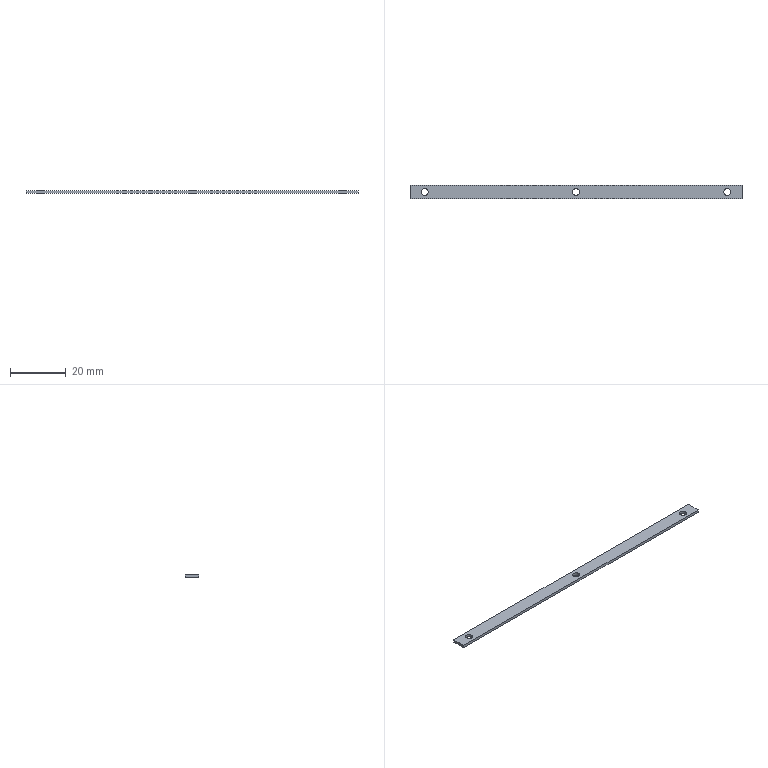Part | SolidWorks | features Cut 1, Extrusion 1 | 1 solid | 12 faces | box 119.31 x 4.994 x 1 mm | volume 581.134 mm3 | cylinder 6 | plane 6 | commonest cylinder face diameters 2.5 x6
STEP:
#1=CARTESIAN_POINT('',(-55.55,59.584,0.));
#2=VERTEX_POINT('',#1);
#3=CARTESIAN_POINT('',(-53.05,59.584,0.));
#4=VERTEX_POINT('',#3);
#5=CARTESIAN_POINT('',(-54.3,59.584,0.));
#6=DIRECTION('',(0.,0.,1.));
#7=DIRECTION('',(1.,0.,0.));
#8=AXIS2_PLACEMENT_3D('',#5,#6,#7);
#9=CIRCLE('',#8,1.25);
#10=EDGE_CURVE('',#2,#4,#9,.T.);
#11=ORIENTED_EDGE('',*,*,#10,.F.);
#12=CARTESIAN_POINT('',(-55.55,59.584,1.));
#13=VERTEX_POINT('',#12);
#14=CARTESIAN_POINT('',(-55.55,59.584,0.));
#15=DIRECTION('',(0.,0.,1.));
#16=VECTOR('',#15,1000.);
#17=LINE('',#14,#16);
#18=EDGE_CURVE('',#2,#13,#17,.T.);
#19=ORIENTED_EDGE('',*,*,#18,.T.);
#20=CARTESIAN_POINT('',(-53.05,59.584,1.));
#21=VERTEX_POINT('',#20);
#22=CARTESIAN_POINT('',(-54.3,59.584,1.));
#23=DIRECTION('',(0.,0.,1.));
#24=DIRECTION('',(1.,0.,0.));
#25=AXIS2_PLACEMENT_3D('',#22,#23,#24);
#26=CIRCLE('',#25,1.25);
#27=EDGE_CURVE('',#13,#21,#26,.T.);
#28=ORIENTED_EDGE('',*,*,#27,.T.);
#29=CARTESIAN_POINT('',(-53.05,59.584,0.));
#30=DIRECTION('',(0.,0.,1.));
#31=VECTOR('',#30,1000.);
#32=LINE('',#29,#31);
#33=EDGE_CURVE('',#4,#21,#32,.T.);
#34=ORIENTED_EDGE('',*,*,#33,.F.);
#35=EDGE_LOOP('',(#11,#19,#28,#34));
#36=FACE_OUTER_BOUND('',#35,.T.);
#37=CARTESIAN_POINT('',(-54.3,59.584,0.));
#38=DIRECTION('',(0.,0.,1.));
#39=DIRECTION('',(1.,0.,0.));
#40=AXIS2_PLACEMENT_3D('',#37,#38,#39);
#41=CYLINDRICAL_SURFACE('',#40,1.25);
#42=ADVANCED_FACE('',(#36),#41,.F.);
#43=CARTESIAN_POINT('',(-1.25,59.56,0.));
#44=VERTEX_POINT('',#43);
#45=CARTESIAN_POINT('',(1.25,59.56,0.));
#46=VERTEX_POINT('',#45);
#47=CARTESIAN_POINT('',(0.,59.56,0.));
#48=DIRECTION('',(0.,0.,1.));
#49=DIRECTION('',(1.,0.,0.));
#50=AXIS2_PLACEMENT_3D('',#47,#48,#49);
#51=CIRCLE('',#50,1.25);
#52=EDGE_CURVE('',#44,#46,#51,.T.);
#53=ORIENTED_EDGE('',*,*,#52,.F.);
#54=CARTESIAN_POINT('',(-1.25,59.56,1.));
#55=VERTEX_POINT('',#54);
#56=CARTESIAN_POINT('',(-1.25,59.56,0.));
#57=DIRECTION('',(0.,0.,1.));
#58=VECTOR('',#57,1000.);
#59=LINE('',#56,#58);
#60=EDGE_CURVE('',#44,#55,#59,.T.);
#61=ORIENTED_EDGE('',*,*,#60,.T.);
#62=CARTESIAN_POINT('',(1.25,59.56,1.));
#63=VERTEX_POINT('',#62);
#64=CARTESIAN_POINT('',(0.,59.56,1.));
#65=DIRECTION('',(0.,0.,1.));
#66=DIRECTION('',(1.,0.,0.));
#67=AXIS2_PLACEMENT_3D('',#64,#65,#66);
#68=CIRCLE('',#67,1.25);
#69=EDGE_CURVE('',#55,#63,#68,.T.);
#70=ORIENTED_EDGE('',*,*,#69,.T.);
#71=CARTESIAN_POINT('',(1.25,59.56,0.));
#72=DIRECTION('',(0.,0.,1.));
#73=VECTOR('',#72,1000.);
#74=LINE('',#71,#73);
#75=EDGE_CURVE('',#46,#63,#74,.T.);
#76=ORIENTED_EDGE('',*,*,#75,.F.);
#77=EDGE_LOOP('',(#53,#61,#70,#76));
#78=FACE_OUTER_BOUND('',#77,.T.);
#79=CARTESIAN_POINT('',(0.,59.56,0.));
#80=DIRECTION('',(0.,0.,1.));
#81=DIRECTION('',(1.,0.,0.));
#82=AXIS2_PLACEMENT_3D('',#79,#80,#81);
#83=CYLINDRICAL_SURFACE('',#82,1.25);
#84=ADVANCED_FACE('',(#78),#83,.F.);
#85=CARTESIAN_POINT('',(53.05,59.584,0.));
#86=VERTEX_POINT('',#85);
#87=CARTESIAN_POINT('',(55.55,59.584,0.));
#88=VERTEX_POINT('',#87);
#89=CARTESIAN_POINT('',(54.3,59.584,0.));
#90=DIRECTION('',(0.,0.,1.));
#91=DIRECTION('',(1.,0.,0.));
#92=AXIS2_PLACEMENT_3D('',#89,#90,#91);
#93=CIRCLE('',#92,1.25);
#94=EDGE_CURVE('',#86,#88,#93,.T.);
#95=ORIENTED_EDGE('',*,*,#94,.F.);
#96=CARTESIAN_POINT('',(53.05,59.584,1.));
#97=VERTEX_POINT('',#96);
#98=CARTESIAN_POINT('',(53.05,59.584,0.));
#99=DIRECTION('',(0.,0.,1.));
#100=VECTOR('',#99,1000.);
#101=LINE('',#98,#100);
#102=EDGE_CURVE('',#86,#97,#101,.T.);
#103=ORIENTED_EDGE('',*,*,#102,.T.);
#104=CARTESIAN_POINT('',(55.55,59.584,1.));
#105=VERTEX_POINT('',#104);
#106=CARTESIAN_POINT('',(54.3,59.584,1.));
#107=DIRECTION('',(0.,0.,1.));
#108=DIRECTION('',(1.,0.,0.));
#109=AXIS2_PLACEMENT_3D('',#106,#107,#108);
#110=CIRCLE('',#109,1.25);
#111=EDGE_CURVE('',#97,#105,#110,.T.);
#112=ORIENTED_EDGE('',*,*,#111,.T.);
#113=CARTESIAN_POINT('',(55.55,59.584,0.));
#114=DIRECTION('',(0.,0.,1.));
#115=VECTOR('',#114,1000.);
#116=LINE('',#113,#115);
#117=EDGE_CURVE('',#88,#105,#116,.T.);
#118=ORIENTED_EDGE('',*,*,#117,.F.);
#119=EDGE_LOOP('',(#95,#103,#112,#118));
#120=FACE_OUTER_BOUND('',#119,.T.);
#121=CARTESIAN_POINT('',(54.3,59.584,0.));
#122=DIRECTION('',(0.,0.,1.));
#123=DIRECTION('',(1.,0.,0.));
#124=AXIS2_PLACEMENT_3D('',#121,#122,#123);
#125=CYLINDRICAL_SURFACE('',#124,1.25);
#126=ADVANCED_FACE('',(#120),#125,.F.);
#127=CARTESIAN_POINT('',(-59.655,62.081,0.));
#128=VERTEX_POINT('',#127);
#129=CARTESIAN_POINT('',(-59.655,57.086,0.));
#130=VERTEX_POINT('',#129);
#131=CARTESIAN_POINT('',(-59.655,62.081,0.));
#132=DIRECTION('',(0.,-1.,0.));
#133=VECTOR('',#132,1000.);
#134=LINE('',#131,#133);
#135=EDGE_CURVE('',#128,#130,#134,.T.);
#136=ORIENTED_EDGE('',*,*,#135,.T.);
#137=CARTESIAN_POINT('',(-59.655,57.086,1.));
#138=VERTEX_POINT('',#137);
#139=CARTESIAN_POINT('',(-59.655,57.086,1.));
#140=DIRECTION('',(0.,0.,-1.));
#141=VECTOR('',#140,1000.);
#142=LINE('',#139,#141);
#143=EDGE_CURVE('',#138,#130,#142,.T.);
#144=ORIENTED_EDGE('',*,*,#143,.F.);
#145=CARTESIAN_POINT('',(-59.655,62.081,1.));
#146=VERTEX_POINT('',#145);
#147=CARTESIAN_POINT('',(-59.655,62.081,1.));
#148=DIRECTION('',(0.,-1.,0.));
#149=VECTOR('',#148,1000.);
#150=LINE('',#147,#149);
#151=EDGE_CURVE('',#146,#138,#150,.T.);
#152=ORIENTED_EDGE('',*,*,#151,.F.);
#153=CARTESIAN_POINT('',(-59.655,62.081,1.));
#154=DIRECTION('',(0.,0.,-1.));
#155=VECTOR('',#154,1000.);
#156=LINE('',#153,#155);
#157=EDGE_CURVE('',#146,#128,#156,.T.);
#158=ORIENTED_EDGE('',*,*,#157,.T.);
#159=EDGE_LOOP('',(#136,#144,#152,#158));
#160=FACE_OUTER_BOUND('',#159,.T.);
#161=CARTESIAN_POINT('',(-59.655,62.081,1.));
#162=DIRECTION('',(1.,0.,0.));
#163=DIRECTION('',(0.,0.,-1.));
#164=AXIS2_PLACEMENT_3D('',#161,#162,#163);
#165=PLANE('',#164);
#166=ADVANCED_FACE('',(#160),#165,.F.);
#167=CARTESIAN_POINT('',(59.655,57.086,0.));
#168=VERTEX_POINT('',#167);
#169=CARTESIAN_POINT('',(59.655,57.086,0.));
#170=DIRECTION('',(1.,0.,0.));
#171=VECTOR('',#170,1000.);
#172=LINE('',#169,#171);
#173=EDGE_CURVE('',#130,#168,#172,.T.);
#174=ORIENTED_EDGE('',*,*,#173,.T.);
#175=CARTESIAN_POINT('',(59.655,57.086,1.));
#176=VERTEX_POINT('',#175);
#177=CARTESIAN_POINT('',(59.655,57.086,1.));
#178=DIRECTION('',(0.,0.,-1.));
#179=VECTOR('',#178,1000.);
#180=LINE('',#177,#179);
#181=EDGE_CURVE('',#176,#168,#180,.T.);
#182=ORIENTED_EDGE('',*,*,#181,.F.);
#183=CARTESIAN_POINT('',(59.655,57.086,1.));
#184=DIRECTION('',(1.,0.,0.));
#185=VECTOR('',#184,1000.);
#186=LINE('',#183,#185);
#187=EDGE_CURVE('',#138,#176,#186,.T.);
#188=ORIENTED_EDGE('',*,*,#187,.F.);
#189=ORIENTED_EDGE('',*,*,#143,.T.);
#190=EDGE_LOOP('',(#174,#182,#188,#189));
#191=FACE_OUTER_BOUND('',#190,.T.);
#192=CARTESIAN_POINT('',(59.655,57.086,1.));
#193=DIRECTION('',(0.,1.,0.));
#194=DIRECTION('',(0.,0.,1.));
#195=AXIS2_PLACEMENT_3D('',#192,#193,#194);
#196=PLANE('',#195);
#197=ADVANCED_FACE('',(#191),#196,.F.);
#198=CARTESIAN_POINT('',(59.655,62.081,0.));
#199=VERTEX_POINT('',#198);
#200=CARTESIAN_POINT('',(59.655,62.081,0.));
#201=DIRECTION('',(0.,1.,0.));
#202=VECTOR('',#201,1000.);
#203=LINE('',#200,#202);
#204=EDGE_CURVE('',#168,#199,#203,.T.);
#205=ORIENTED_EDGE('',*,*,#204,.T.);
#206=CARTESIAN_POINT('',(59.655,62.081,1.));
#207=VERTEX_POINT('',#206);
#208=CARTESIAN_POINT('',(59.655,62.081,1.));
#209=DIRECTION('',(0.,0.,-1.));
#210=VECTOR('',#209,1000.);
#211=LINE('',#208,#210);
#212=EDGE_CURVE('',#207,#199,#211,.T.);
#213=ORIENTED_EDGE('',*,*,#212,.F.);
#214=CARTESIAN_POINT('',(59.655,62.081,1.));
#215=DIRECTION('',(0.,1.,0.));
#216=VECTOR('',#215,1000.);
#217=LINE('',#214,#216);
#218=EDGE_CURVE('',#176,#207,#217,.T.);
#219=ORIENTED_EDGE('',*,*,#218,.F.);
#220=ORIENTED_EDGE('',*,*,#181,.T.);
#221=EDGE_LOOP('',(#205,#213,#219,#220));
#222=FACE_OUTER_BOUND('',#221,.T.);
#223=CARTESIAN_POINT('',(59.655,62.081,1.));
#224=DIRECTION('',(-1.,0.,0.));
#225=DIRECTION('',(0.,0.,1.));
#226=AXIS2_PLACEMENT_3D('',#223,#224,#225);
#227=PLANE('',#226);
#228=ADVANCED_FACE('',(#222),#227,.F.);
#229=CARTESIAN_POINT('',(59.655,62.081,0.));
#230=DIRECTION('',(-1.,0.,0.));
#231=VECTOR('',#230,1000.);
#232=LINE('',#229,#231);
#233=EDGE_CURVE('',#199,#128,#232,.T.);
#234=ORIENTED_EDGE('',*,*,#233,.T.);
#235=ORIENTED_EDGE('',*,*,#157,.F.);
#236=CARTESIAN_POINT('',(59.655,62.081,1.));
#237=DIRECTION('',(-1.,0.,0.));
#238=VECTOR('',#237,1000.);
#239=LINE('',#236,#238);
#240=EDGE_CURVE('',#207,#146,#239,.T.);
#241=ORIENTED_EDGE('',*,*,#240,.F.);
#242=ORIENTED_EDGE('',*,*,#212,.T.);
#243=EDGE_LOOP('',(#234,#235,#241,#242));
#244=FACE_OUTER_BOUND('',#243,.T.);
#245=CARTESIAN_POINT('',(59.655,62.081,1.));
#246=DIRECTION('',(0.,-1.,0.));
#247=DIRECTION('',(0.,0.,-1.));
#248=AXIS2_PLACEMENT_3D('',#245,#246,#247);
#249=PLANE('',#248);
#250=ADVANCED_FACE('',(#244),#249,.F.);
#251=CARTESIAN_POINT('',(-54.3,59.584,1.));
#252=DIRECTION('',(0.,0.,1.));
#253=DIRECTION('',(1.,0.,0.));
#254=AXIS2_PLACEMENT_3D('',#251,#252,#253);
#255=CIRCLE('',#254,1.25);
#256=EDGE_CURVE('',#21,#13,#255,.T.);
#257=ORIENTED_EDGE('',*,*,#256,.F.);
#258=ORIENTED_EDGE('',*,*,#27,.F.);
#259=EDGE_LOOP('',(#257,#258));
#260=FACE_BOUND('',#259,.T.);
#261=CARTESIAN_POINT('',(0.,59.56,1.));
#262=DIRECTION('',(0.,0.,1.));
#263=DIRECTION('',(1.,0.,0.));
#264=AXIS2_PLACEMENT_3D('',#261,#262,#263);
#265=CIRCLE('',#264,1.25);
#266=EDGE_CURVE('',#63,#55,#265,.T.);
#267=ORIENTED_EDGE('',*,*,#266,.F.);
#268=ORIENTED_EDGE('',*,*,#69,.F.);
#269=EDGE_LOOP('',(#267,#268));
#270=FACE_BOUND('',#269,.T.);
#271=CARTESIAN_POINT('',(54.3,59.584,1.));
#272=DIRECTION('',(0.,0.,1.));
#273=DIRECTION('',(1.,0.,0.));
#274=AXIS2_PLACEMENT_3D('',#271,#272,#273);
#275=CIRCLE('',#274,1.25);
#276=EDGE_CURVE('',#105,#97,#275,.T.);
#277=ORIENTED_EDGE('',*,*,#276,.F.);
#278=ORIENTED_EDGE('',*,*,#111,.F.);
#279=EDGE_LOOP('',(#277,#278));
#280=FACE_BOUND('',#279,.T.);
#281=ORIENTED_EDGE('',*,*,#151,.T.);
#282=ORIENTED_EDGE('',*,*,#187,.T.);
#283=ORIENTED_EDGE('',*,*,#218,.T.);
#284=ORIENTED_EDGE('',*,*,#240,.T.);
#285=EDGE_LOOP('',(#281,#282,#283,#284));
#286=FACE_OUTER_BOUND('',#285,.T.);
#287=CARTESIAN_POINT('',(0.,0.,1.));
#288=DIRECTION('',(0.,0.,-1.));
#289=DIRECTION('',(-1.,0.,0.));
#290=AXIS2_PLACEMENT_3D('',#287,#288,#289);
#291=PLANE('',#290);
#292=ADVANCED_FACE('',(#260,#270,#280,#286),#291,.F.);
#293=CARTESIAN_POINT('',(-54.3,59.584,0.));
#294=DIRECTION('',(0.,0.,1.));
#295=DIRECTION('',(1.,0.,0.));
#296=AXIS2_PLACEMENT_3D('',#293,#294,#295);
#297=CIRCLE('',#296,1.25);
#298=EDGE_CURVE('',#4,#2,#297,.T.);
#299=ORIENTED_EDGE('',*,*,#298,.T.);
#300=ORIENTED_EDGE('',*,*,#10,.T.);
#301=EDGE_LOOP('',(#299,#300));
#302=FACE_BOUND('',#301,.T.);
#303=CARTESIAN_POINT('',(0.,59.56,0.));
#304=DIRECTION('',(0.,0.,1.));
#305=DIRECTION('',(1.,0.,0.));
#306=AXIS2_PLACEMENT_3D('',#303,#304,#305);
#307=CIRCLE('',#306,1.25);
#308=EDGE_CURVE('',#46,#44,#307,.T.);
#309=ORIENTED_EDGE('',*,*,#308,.T.);
#310=ORIENTED_EDGE('',*,*,#52,.T.);
#311=EDGE_LOOP('',(#309,#310));
#312=FACE_BOUND('',#311,.T.);
#313=CARTESIAN_POINT('',(54.3,59.584,0.));
#314=DIRECTION('',(0.,0.,1.));
#315=DIRECTION('',(1.,0.,0.));
#316=AXIS2_PLACEMENT_3D('',#313,#314,#315);
#317=CIRCLE('',#316,1.25);
#318=EDGE_CURVE('',#88,#86,#317,.T.);
#319=ORIENTED_EDGE('',*,*,#318,.T.);
#320=ORIENTED_EDGE('',*,*,#94,.T.);
#321=EDGE_LOOP('',(#319,#320));
#322=FACE_BOUND('',#321,.T.);
#323=ORIENTED_EDGE('',*,*,#135,.F.);
#324=ORIENTED_EDGE('',*,*,#233,.F.);
#325=ORIENTED_EDGE('',*,*,#204,.F.);
#326=ORIENTED_EDGE('',*,*,#173,.F.);
#327=EDGE_LOOP('',(#323,#324,#325,#326));
#328=FACE_OUTER_BOUND('',#327,.T.);
#329=CARTESIAN_POINT('',(0.,0.,0.));
#330=DIRECTION('',(0.,0.,-1.));
#331=DIRECTION('',(-1.,0.,0.));
#332=AXIS2_PLACEMENT_3D('',#329,#330,#331);
#333=PLANE('',#332);
#334=ADVANCED_FACE('',(#302,#312,#322,#328),#333,.T.);
#335=ORIENTED_EDGE('',*,*,#102,.F.);
#336=ORIENTED_EDGE('',*,*,#318,.F.);
#337=ORIENTED_EDGE('',*,*,#117,.T.);
#338=ORIENTED_EDGE('',*,*,#276,.T.);
#339=EDGE_LOOP('',(#335,#336,#337,#338));
#340=FACE_OUTER_BOUND('',#339,.T.);
#341=CARTESIAN_POINT('',(54.3,59.584,0.));
#342=DIRECTION('',(0.,0.,1.));
#343=DIRECTION('',(1.,0.,0.));
#344=AXIS2_PLACEMENT_3D('',#341,#342,#343);
#345=CYLINDRICAL_SURFACE('',#344,1.25);
#346=ADVANCED_FACE('',(#340),#345,.F.);
#347=ORIENTED_EDGE('',*,*,#60,.F.);
#348=ORIENTED_EDGE('',*,*,#308,.F.);
#349=ORIENTED_EDGE('',*,*,#75,.T.);
#350=ORIENTED_EDGE('',*,*,#266,.T.);
#351=EDGE_LOOP('',(#347,#348,#349,#350));
#352=FACE_OUTER_BOUND('',#351,.T.);
#353=CARTESIAN_POINT('',(0.,59.56,0.));
#354=DIRECTION('',(0.,0.,1.));
#355=DIRECTION('',(1.,0.,0.));
#356=AXIS2_PLACEMENT_3D('',#353,#354,#355);
#357=CYLINDRICAL_SURFACE('',#356,1.25);
#358=ADVANCED_FACE('',(#352),#357,.F.);
#359=ORIENTED_EDGE('',*,*,#18,.F.);
#360=ORIENTED_EDGE('',*,*,#298,.F.);
#361=ORIENTED_EDGE('',*,*,#33,.T.);
#362=ORIENTED_EDGE('',*,*,#256,.T.);
#363=EDGE_LOOP('',(#359,#360,#361,#362));
#364=FACE_OUTER_BOUND('',#363,.T.);
#365=CARTESIAN_POINT('',(-54.3,59.584,0.));
#366=DIRECTION('',(0.,0.,1.));
#367=DIRECTION('',(1.,0.,0.));
#368=AXIS2_PLACEMENT_3D('',#365,#366,#367);
#369=CYLINDRICAL_SURFACE('',#368,1.25);
#370=ADVANCED_FACE('',(#364),#369,.F.);
#371=CLOSED_SHELL('',(#42,#84,#126,#166,#197,#228,#250,#292,#334,#346,#358,#370));
#372=MANIFOLD_SOLID_BREP('',#371);
#373=CARTESIAN_POINT('',(0.,0.,0.));
#374=DIRECTION('',(0.,0.,1.));
#375=DIRECTION('',(1.,0.,0.));
#376=AXIS2_PLACEMENT_3D('',#373,#374,#375);
#377=(LENGTH_UNIT()NAMED_UNIT(*)SI_UNIT(.MILLI.,.METRE.));
#378=UNCERTAINTY_MEASURE_WITH_UNIT(LENGTH_MEASURE(0.00001),#377,'','');
#379=(NAMED_UNIT(*)PLANE_ANGLE_UNIT()SI_UNIT($,.RADIAN.));
#380=(NAMED_UNIT(*)SI_UNIT($,.STERADIAN.)SOLID_ANGLE_UNIT());
#381=(GEOMETRIC_REPRESENTATION_CONTEXT(3)GLOBAL_UNCERTAINTY_ASSIGNED_CONTEXT((#378))GLOBAL_UNIT_ASSIGNED_CONTEXT((#377,#379,#380))REPRESENTATION_CONTEXT('',''));
#382=ADVANCED_BREP_SHAPE_REPRESENTATION('',(#372,#376),#381);